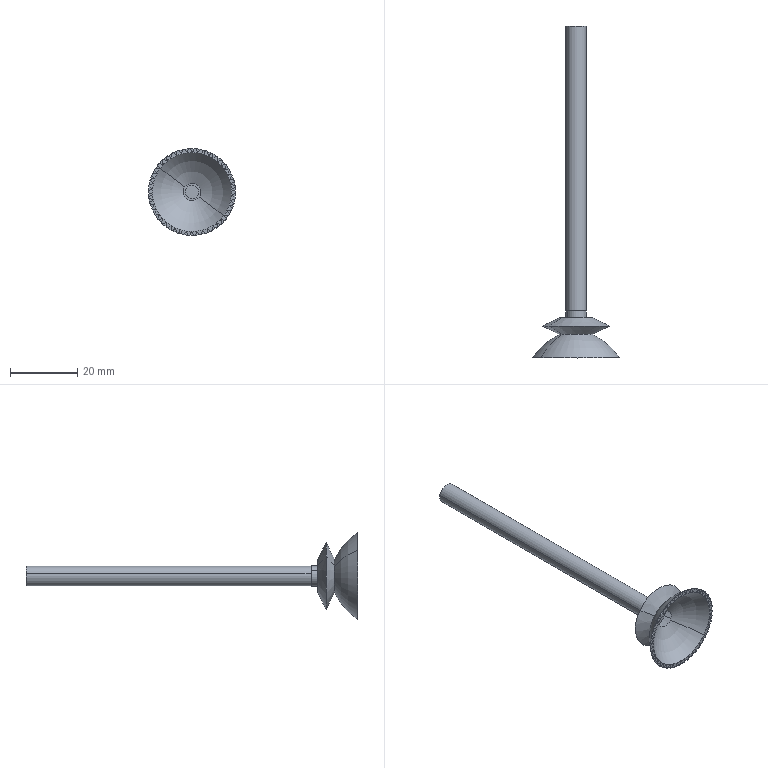Part | SolidWorks | 2 solids | 208 faces | box 26 x 99 x 25.974 mm | volume 3520 mm3 | plane 190 | cone 8 | cylinder 6 | torus 4 | commonest cylinder face diameters 6 x4 4 x2